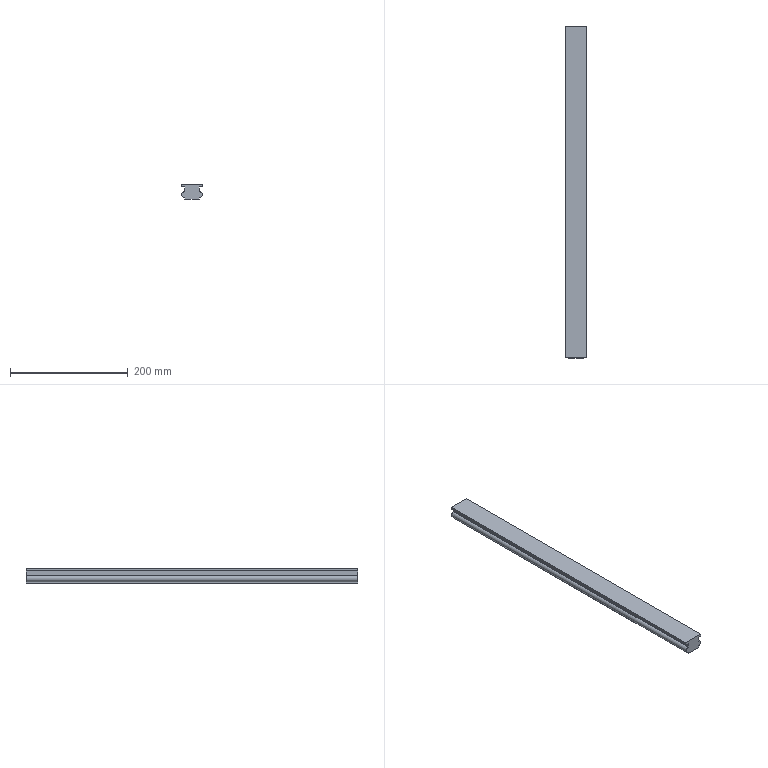Part | SolidWorks | features Extrusion 1 | 1 solid | 14 faces | box 36 x 563 x 25 mm | volume 420865 mm3 | plane 12 | cylinder 2 | commonest cylinder face diameters 10 x2
STEP:
#1=CARTESIAN_POINT('',(12.5,0.,5.));
#2=VERTEX_POINT('',#1);
#3=CARTESIAN_POINT('',(12.5,0.,-5.));
#4=VERTEX_POINT('',#3);
#5=CARTESIAN_POINT('',(12.5,0.,0.));
#6=DIRECTION('',(0.,1.,0.));
#7=DIRECTION('',(0.,0.,1.));
#8=AXIS2_PLACEMENT_3D('',#5,#6,#7);
#9=CIRCLE('',#8,5.);
#10=EDGE_CURVE('',#2,#4,#9,.T.);
#11=ORIENTED_EDGE('',*,*,#10,.T.);
#12=CARTESIAN_POINT('',(12.5,563.,-5.));
#13=VERTEX_POINT('',#12);
#14=CARTESIAN_POINT('',(12.5,563.,-5.));
#15=DIRECTION('',(0.,-1.,0.));
#16=VECTOR('',#15,1000.);
#17=LINE('',#14,#16);
#18=EDGE_CURVE('',#13,#4,#17,.T.);
#19=ORIENTED_EDGE('',*,*,#18,.F.);
#20=CARTESIAN_POINT('',(12.5,563.,5.));
#21=VERTEX_POINT('',#20);
#22=CARTESIAN_POINT('',(12.5,563.,0.));
#23=DIRECTION('',(0.,1.,0.));
#24=DIRECTION('',(0.,0.,1.));
#25=AXIS2_PLACEMENT_3D('',#22,#23,#24);
#26=CIRCLE('',#25,5.);
#27=EDGE_CURVE('',#21,#13,#26,.T.);
#28=ORIENTED_EDGE('',*,*,#27,.F.);
#29=CARTESIAN_POINT('',(12.5,563.,5.));
#30=DIRECTION('',(0.,-1.,0.));
#31=VECTOR('',#30,1000.);
#32=LINE('',#29,#31);
#33=EDGE_CURVE('',#21,#2,#32,.T.);
#34=ORIENTED_EDGE('',*,*,#33,.T.);
#35=EDGE_LOOP('',(#11,#19,#28,#34));
#36=FACE_OUTER_BOUND('',#35,.T.);
#37=CARTESIAN_POINT('',(12.5,563.,0.));
#38=DIRECTION('',(0.,-1.,0.));
#39=DIRECTION('',(0.,0.,-1.));
#40=AXIS2_PLACEMENT_3D('',#37,#38,#39);
#41=CYLINDRICAL_SURFACE('',#40,5.);
#42=ADVANCED_FACE('',(#36),#41,.T.);
#43=CARTESIAN_POINT('',(12.5,0.,-8.));
#44=VERTEX_POINT('',#43);
#45=CARTESIAN_POINT('',(12.5,0.,-8.));
#46=DIRECTION('',(0.,0.,-1.));
#47=VECTOR('',#46,1000.);
#48=LINE('',#45,#47);
#49=EDGE_CURVE('',#4,#44,#48,.T.);
#50=ORIENTED_EDGE('',*,*,#49,.T.);
#51=CARTESIAN_POINT('',(12.5,563.,-8.));
#52=VERTEX_POINT('',#51);
#53=CARTESIAN_POINT('',(12.5,563.,-8.));
#54=DIRECTION('',(0.,-1.,0.));
#55=VECTOR('',#54,1000.);
#56=LINE('',#53,#55);
#57=EDGE_CURVE('',#52,#44,#56,.T.);
#58=ORIENTED_EDGE('',*,*,#57,.F.);
#59=CARTESIAN_POINT('',(12.5,563.,-8.));
#60=DIRECTION('',(0.,0.,-1.));
#61=VECTOR('',#60,1000.);
#62=LINE('',#59,#61);
#63=EDGE_CURVE('',#13,#52,#62,.T.);
#64=ORIENTED_EDGE('',*,*,#63,.F.);
#65=ORIENTED_EDGE('',*,*,#18,.T.);
#66=EDGE_LOOP('',(#50,#58,#64,#65));
#67=FACE_OUTER_BOUND('',#66,.T.);
#68=CARTESIAN_POINT('',(12.5,563.,-8.));
#69=DIRECTION('',(-1.,0.,0.));
#70=DIRECTION('',(0.,0.,1.));
#71=AXIS2_PLACEMENT_3D('',#68,#69,#70);
#72=PLANE('',#71);
#73=ADVANCED_FACE('',(#67),#72,.F.);
#74=CARTESIAN_POINT('',(-12.5,0.,-8.));
#75=VERTEX_POINT('',#74);
#76=CARTESIAN_POINT('',(-12.5,0.,-8.));
#77=DIRECTION('',(-1.,0.,0.));
#78=VECTOR('',#77,1000.);
#79=LINE('',#76,#78);
#80=EDGE_CURVE('',#44,#75,#79,.T.);
#81=ORIENTED_EDGE('',*,*,#80,.T.);
#82=CARTESIAN_POINT('',(-12.5,563.,-8.));
#83=VERTEX_POINT('',#82);
#84=CARTESIAN_POINT('',(-12.5,563.,-8.));
#85=DIRECTION('',(0.,-1.,0.));
#86=VECTOR('',#85,1000.);
#87=LINE('',#84,#86);
#88=EDGE_CURVE('',#83,#75,#87,.T.);
#89=ORIENTED_EDGE('',*,*,#88,.F.);
#90=CARTESIAN_POINT('',(-12.5,563.,-8.));
#91=DIRECTION('',(-1.,0.,0.));
#92=VECTOR('',#91,1000.);
#93=LINE('',#90,#92);
#94=EDGE_CURVE('',#52,#83,#93,.T.);
#95=ORIENTED_EDGE('',*,*,#94,.F.);
#96=ORIENTED_EDGE('',*,*,#57,.T.);
#97=EDGE_LOOP('',(#81,#89,#95,#96));
#98=FACE_OUTER_BOUND('',#97,.T.);
#99=CARTESIAN_POINT('',(-12.5,563.,-8.));
#100=DIRECTION('',(0.,0.,1.));
#101=DIRECTION('',(1.,0.,0.));
#102=AXIS2_PLACEMENT_3D('',#99,#100,#101);
#103=PLANE('',#102);
#104=ADVANCED_FACE('',(#98),#103,.F.);
#105=CARTESIAN_POINT('',(-12.5,0.,-5.));
#106=VERTEX_POINT('',#105);
#107=CARTESIAN_POINT('',(-12.5,0.,-5.));
#108=DIRECTION('',(0.,0.,1.));
#109=VECTOR('',#108,1000.);
#110=LINE('',#107,#109);
#111=EDGE_CURVE('',#75,#106,#110,.T.);
#112=ORIENTED_EDGE('',*,*,#111,.T.);
#113=CARTESIAN_POINT('',(-12.5,563.,-5.));
#114=VERTEX_POINT('',#113);
#115=CARTESIAN_POINT('',(-12.5,563.,-5.));
#116=DIRECTION('',(0.,-1.,0.));
#117=VECTOR('',#116,1000.);
#118=LINE('',#115,#117);
#119=EDGE_CURVE('',#114,#106,#118,.T.);
#120=ORIENTED_EDGE('',*,*,#119,.F.);
#121=CARTESIAN_POINT('',(-12.5,563.,-5.));
#122=DIRECTION('',(0.,0.,1.));
#123=VECTOR('',#122,1000.);
#124=LINE('',#121,#123);
#125=EDGE_CURVE('',#83,#114,#124,.T.);
#126=ORIENTED_EDGE('',*,*,#125,.F.);
#127=ORIENTED_EDGE('',*,*,#88,.T.);
#128=EDGE_LOOP('',(#112,#120,#126,#127));
#129=FACE_OUTER_BOUND('',#128,.T.);
#130=CARTESIAN_POINT('',(-12.5,563.,-5.));
#131=DIRECTION('',(1.,0.,0.));
#132=DIRECTION('',(0.,0.,-1.));
#133=AXIS2_PLACEMENT_3D('',#130,#131,#132);
#134=PLANE('',#133);
#135=ADVANCED_FACE('',(#129),#134,.F.);
#136=CARTESIAN_POINT('',(-12.5,0.,5.));
#137=VERTEX_POINT('',#136);
#138=CARTESIAN_POINT('',(-12.5,0.,0.));
#139=DIRECTION('',(0.,1.,0.));
#140=DIRECTION('',(0.,0.,1.));
#141=AXIS2_PLACEMENT_3D('',#138,#139,#140);
#142=CIRCLE('',#141,5.);
#143=EDGE_CURVE('',#106,#137,#142,.T.);
#144=ORIENTED_EDGE('',*,*,#143,.T.);
#145=CARTESIAN_POINT('',(-12.5,563.,5.));
#146=VERTEX_POINT('',#145);
#147=CARTESIAN_POINT('',(-12.5,563.,5.));
#148=DIRECTION('',(0.,-1.,0.));
#149=VECTOR('',#148,1000.);
#150=LINE('',#147,#149);
#151=EDGE_CURVE('',#146,#137,#150,.T.);
#152=ORIENTED_EDGE('',*,*,#151,.F.);
#153=CARTESIAN_POINT('',(-12.5,563.,0.));
#154=DIRECTION('',(0.,1.,0.));
#155=DIRECTION('',(0.,0.,1.));
#156=AXIS2_PLACEMENT_3D('',#153,#154,#155);
#157=CIRCLE('',#156,5.);
#158=EDGE_CURVE('',#114,#146,#157,.T.);
#159=ORIENTED_EDGE('',*,*,#158,.F.);
#160=ORIENTED_EDGE('',*,*,#119,.T.);
#161=EDGE_LOOP('',(#144,#152,#159,#160));
#162=FACE_OUTER_BOUND('',#161,.T.);
#163=CARTESIAN_POINT('',(-12.5,563.,0.));
#164=DIRECTION('',(0.,-1.,0.));
#165=DIRECTION('',(0.,0.,-1.));
#166=AXIS2_PLACEMENT_3D('',#163,#164,#165);
#167=CYLINDRICAL_SURFACE('',#166,5.);
#168=ADVANCED_FACE('',(#162),#167,.T.);
#169=CARTESIAN_POINT('',(-12.5,0.,13.));
#170=VERTEX_POINT('',#169);
#171=CARTESIAN_POINT('',(-12.5,0.,5.));
#172=DIRECTION('',(0.,0.,1.));
#173=VECTOR('',#172,1000.);
#174=LINE('',#171,#173);
#175=EDGE_CURVE('',#137,#170,#174,.T.);
#176=ORIENTED_EDGE('',*,*,#175,.T.);
#177=CARTESIAN_POINT('',(-12.5,563.,13.));
#178=VERTEX_POINT('',#177);
#179=CARTESIAN_POINT('',(-12.5,563.,13.));
#180=DIRECTION('',(0.,-1.,0.));
#181=VECTOR('',#180,1000.);
#182=LINE('',#179,#181);
#183=EDGE_CURVE('',#178,#170,#182,.T.);
#184=ORIENTED_EDGE('',*,*,#183,.F.);
#185=CARTESIAN_POINT('',(-12.5,563.,5.));
#186=DIRECTION('',(0.,0.,1.));
#187=VECTOR('',#186,1000.);
#188=LINE('',#185,#187);
#189=EDGE_CURVE('',#146,#178,#188,.T.);
#190=ORIENTED_EDGE('',*,*,#189,.F.);
#191=ORIENTED_EDGE('',*,*,#151,.T.);
#192=EDGE_LOOP('',(#176,#184,#190,#191));
#193=FACE_OUTER_BOUND('',#192,.T.);
#194=CARTESIAN_POINT('',(-12.5,563.,5.));
#195=DIRECTION('',(1.,0.,0.));
#196=DIRECTION('',(0.,0.,-1.));
#197=AXIS2_PLACEMENT_3D('',#194,#195,#196);
#198=PLANE('',#197);
#199=ADVANCED_FACE('',(#193),#198,.F.);
#200=CARTESIAN_POINT('',(-18.,0.,13.));
#201=VERTEX_POINT('',#200);
#202=CARTESIAN_POINT('',(-12.5,0.,13.));
#203=DIRECTION('',(-1.,0.,0.));
#204=VECTOR('',#203,1000.);
#205=LINE('',#202,#204);
#206=EDGE_CURVE('',#170,#201,#205,.T.);
#207=ORIENTED_EDGE('',*,*,#206,.T.);
#208=CARTESIAN_POINT('',(-18.,563.,13.));
#209=VERTEX_POINT('',#208);
#210=CARTESIAN_POINT('',(-18.,563.,13.));
#211=DIRECTION('',(0.,-1.,0.));
#212=VECTOR('',#211,1000.);
#213=LINE('',#210,#212);
#214=EDGE_CURVE('',#209,#201,#213,.T.);
#215=ORIENTED_EDGE('',*,*,#214,.F.);
#216=CARTESIAN_POINT('',(-12.5,563.,13.));
#217=DIRECTION('',(-1.,0.,0.));
#218=VECTOR('',#217,1000.);
#219=LINE('',#216,#218);
#220=EDGE_CURVE('',#178,#209,#219,.T.);
#221=ORIENTED_EDGE('',*,*,#220,.F.);
#222=ORIENTED_EDGE('',*,*,#183,.T.);
#223=EDGE_LOOP('',(#207,#215,#221,#222));
#224=FACE_OUTER_BOUND('',#223,.T.);
#225=CARTESIAN_POINT('',(-12.5,563.,13.));
#226=DIRECTION('',(0.,0.,1.));
#227=DIRECTION('',(1.,0.,0.));
#228=AXIS2_PLACEMENT_3D('',#225,#226,#227);
#229=PLANE('',#228);
#230=ADVANCED_FACE('',(#224),#229,.F.);
#231=CARTESIAN_POINT('',(-18.,0.,17.));
#232=VERTEX_POINT('',#231);
#233=CARTESIAN_POINT('',(-18.,0.,13.));
#234=DIRECTION('',(0.,0.,1.));
#235=VECTOR('',#234,1000.);
#236=LINE('',#233,#235);
#237=EDGE_CURVE('',#201,#232,#236,.T.);
#238=ORIENTED_EDGE('',*,*,#237,.T.);
#239=CARTESIAN_POINT('',(-18.,563.,17.));
#240=VERTEX_POINT('',#239);
#241=CARTESIAN_POINT('',(-18.,563.,17.));
#242=DIRECTION('',(0.,-1.,0.));
#243=VECTOR('',#242,1000.);
#244=LINE('',#241,#243);
#245=EDGE_CURVE('',#240,#232,#244,.T.);
#246=ORIENTED_EDGE('',*,*,#245,.F.);
#247=CARTESIAN_POINT('',(-18.,563.,13.));
#248=DIRECTION('',(0.,0.,1.));
#249=VECTOR('',#248,1000.);
#250=LINE('',#247,#249);
#251=EDGE_CURVE('',#209,#240,#250,.T.);
#252=ORIENTED_EDGE('',*,*,#251,.F.);
#253=ORIENTED_EDGE('',*,*,#214,.T.);
#254=EDGE_LOOP('',(#238,#246,#252,#253));
#255=FACE_OUTER_BOUND('',#254,.T.);
#256=CARTESIAN_POINT('',(-18.,563.,13.));
#257=DIRECTION('',(1.,0.,0.));
#258=DIRECTION('',(0.,0.,-1.));
#259=AXIS2_PLACEMENT_3D('',#256,#257,#258);
#260=PLANE('',#259);
#261=ADVANCED_FACE('',(#255),#260,.F.);
#262=CARTESIAN_POINT('',(18.,0.,17.));
#263=VERTEX_POINT('',#262);
#264=CARTESIAN_POINT('',(-18.,0.,17.));
#265=DIRECTION('',(1.,0.,0.));
#266=VECTOR('',#265,1000.);
#267=LINE('',#264,#266);
#268=EDGE_CURVE('',#232,#263,#267,.T.);
#269=ORIENTED_EDGE('',*,*,#268,.T.);
#270=CARTESIAN_POINT('',(18.,563.,17.));
#271=VERTEX_POINT('',#270);
#272=CARTESIAN_POINT('',(18.,563.,17.));
#273=DIRECTION('',(0.,-1.,0.));
#274=VECTOR('',#273,1000.);
#275=LINE('',#272,#274);
#276=EDGE_CURVE('',#271,#263,#275,.T.);
#277=ORIENTED_EDGE('',*,*,#276,.F.);
#278=CARTESIAN_POINT('',(-18.,563.,17.));
#279=DIRECTION('',(1.,0.,0.));
#280=VECTOR('',#279,1000.);
#281=LINE('',#278,#280);
#282=EDGE_CURVE('',#240,#271,#281,.T.);
#283=ORIENTED_EDGE('',*,*,#282,.F.);
#284=ORIENTED_EDGE('',*,*,#245,.T.);
#285=EDGE_LOOP('',(#269,#277,#283,#284));
#286=FACE_OUTER_BOUND('',#285,.T.);
#287=CARTESIAN_POINT('',(-18.,563.,17.));
#288=DIRECTION('',(0.,0.,-1.));
#289=DIRECTION('',(-1.,0.,0.));
#290=AXIS2_PLACEMENT_3D('',#287,#288,#289);
#291=PLANE('',#290);
#292=ADVANCED_FACE('',(#286),#291,.F.);
#293=CARTESIAN_POINT('',(18.,0.,13.));
#294=VERTEX_POINT('',#293);
#295=CARTESIAN_POINT('',(18.,0.,17.));
#296=DIRECTION('',(0.,0.,-1.));
#297=VECTOR('',#296,1000.);
#298=LINE('',#295,#297);
#299=EDGE_CURVE('',#263,#294,#298,.T.);
#300=ORIENTED_EDGE('',*,*,#299,.T.);
#301=CARTESIAN_POINT('',(18.,563.,13.));
#302=VERTEX_POINT('',#301);
#303=CARTESIAN_POINT('',(18.,563.,13.));
#304=DIRECTION('',(0.,-1.,0.));
#305=VECTOR('',#304,1000.);
#306=LINE('',#303,#305);
#307=EDGE_CURVE('',#302,#294,#306,.T.);
#308=ORIENTED_EDGE('',*,*,#307,.F.);
#309=CARTESIAN_POINT('',(18.,563.,17.));
#310=DIRECTION('',(0.,0.,-1.));
#311=VECTOR('',#310,1000.);
#312=LINE('',#309,#311);
#313=EDGE_CURVE('',#271,#302,#312,.T.);
#314=ORIENTED_EDGE('',*,*,#313,.F.);
#315=ORIENTED_EDGE('',*,*,#276,.T.);
#316=EDGE_LOOP('',(#300,#308,#314,#315));
#317=FACE_OUTER_BOUND('',#316,.T.);
#318=CARTESIAN_POINT('',(18.,563.,17.));
#319=DIRECTION('',(-1.,0.,0.));
#320=DIRECTION('',(0.,0.,1.));
#321=AXIS2_PLACEMENT_3D('',#318,#319,#320);
#322=PLANE('',#321);
#323=ADVANCED_FACE('',(#317),#322,.F.);
#324=CARTESIAN_POINT('',(12.5,0.,13.));
#325=VERTEX_POINT('',#324);
#326=CARTESIAN_POINT('',(18.,0.,13.));
#327=DIRECTION('',(-1.,0.,0.));
#328=VECTOR('',#327,1000.);
#329=LINE('',#326,#328);
#330=EDGE_CURVE('',#294,#325,#329,.T.);
#331=ORIENTED_EDGE('',*,*,#330,.T.);
#332=CARTESIAN_POINT('',(12.5,563.,13.));
#333=VERTEX_POINT('',#332);
#334=CARTESIAN_POINT('',(12.5,563.,13.));
#335=DIRECTION('',(0.,-1.,0.));
#336=VECTOR('',#335,1000.);
#337=LINE('',#334,#336);
#338=EDGE_CURVE('',#333,#325,#337,.T.);
#339=ORIENTED_EDGE('',*,*,#338,.F.);
#340=CARTESIAN_POINT('',(18.,563.,13.));
#341=DIRECTION('',(-1.,0.,0.));
#342=VECTOR('',#341,1000.);
#343=LINE('',#340,#342);
#344=EDGE_CURVE('',#302,#333,#343,.T.);
#345=ORIENTED_EDGE('',*,*,#344,.F.);
#346=ORIENTED_EDGE('',*,*,#307,.T.);
#347=EDGE_LOOP('',(#331,#339,#345,#346));
#348=FACE_OUTER_BOUND('',#347,.T.);
#349=CARTESIAN_POINT('',(18.,563.,13.));
#350=DIRECTION('',(0.,0.,1.));
#351=DIRECTION('',(1.,0.,0.));
#352=AXIS2_PLACEMENT_3D('',#349,#350,#351);
#353=PLANE('',#352);
#354=ADVANCED_FACE('',(#348),#353,.F.);
#355=CARTESIAN_POINT('',(12.5,0.,13.));
#356=DIRECTION('',(0.,0.,-1.));
#357=VECTOR('',#356,1000.);
#358=LINE('',#355,#357);
#359=EDGE_CURVE('',#325,#2,#358,.T.);
#360=ORIENTED_EDGE('',*,*,#359,.T.);
#361=ORIENTED_EDGE('',*,*,#33,.F.);
#362=CARTESIAN_POINT('',(12.5,563.,13.));
#363=DIRECTION('',(0.,0.,-1.));
#364=VECTOR('',#363,1000.);
#365=LINE('',#362,#364);
#366=EDGE_CURVE('',#333,#21,#365,.T.);
#367=ORIENTED_EDGE('',*,*,#366,.F.);
#368=ORIENTED_EDGE('',*,*,#338,.T.);
#369=EDGE_LOOP('',(#360,#361,#367,#368));
#370=FACE_OUTER_BOUND('',#369,.T.);
#371=CARTESIAN_POINT('',(12.5,563.,13.));
#372=DIRECTION('',(-1.,0.,0.));
#373=DIRECTION('',(0.,0.,1.));
#374=AXIS2_PLACEMENT_3D('',#371,#372,#373);
#375=PLANE('',#374);
#376=ADVANCED_FACE('',(#370),#375,.F.);
#377=ORIENTED_EDGE('',*,*,#27,.T.);
#378=ORIENTED_EDGE('',*,*,#63,.T.);
#379=ORIENTED_EDGE('',*,*,#94,.T.);
#380=ORIENTED_EDGE('',*,*,#125,.T.);
#381=ORIENTED_EDGE('',*,*,#158,.T.);
#382=ORIENTED_EDGE('',*,*,#189,.T.);
#383=ORIENTED_EDGE('',*,*,#220,.T.);
#384=ORIENTED_EDGE('',*,*,#251,.T.);
#385=ORIENTED_EDGE('',*,*,#282,.T.);
#386=ORIENTED_EDGE('',*,*,#313,.T.);
#387=ORIENTED_EDGE('',*,*,#344,.T.);
#388=ORIENTED_EDGE('',*,*,#366,.T.);
#389=EDGE_LOOP('',(#377,#378,#379,#380,#381,#382,#383,#384,#385,#386,#387,#388));
#390=FACE_OUTER_BOUND('',#389,.T.);
#391=CARTESIAN_POINT('',(12.5,563.,0.));
#392=DIRECTION('',(0.,1.,0.));
#393=DIRECTION('',(0.,0.,1.));
#394=AXIS2_PLACEMENT_3D('',#391,#392,#393);
#395=PLANE('',#394);
#396=ADVANCED_FACE('',(#390),#395,.T.);
#397=ORIENTED_EDGE('',*,*,#10,.F.);
#398=ORIENTED_EDGE('',*,*,#359,.F.);
#399=ORIENTED_EDGE('',*,*,#330,.F.);
#400=ORIENTED_EDGE('',*,*,#299,.F.);
#401=ORIENTED_EDGE('',*,*,#268,.F.);
#402=ORIENTED_EDGE('',*,*,#237,.F.);
#403=ORIENTED_EDGE('',*,*,#206,.F.);
#404=ORIENTED_EDGE('',*,*,#175,.F.);
#405=ORIENTED_EDGE('',*,*,#143,.F.);
#406=ORIENTED_EDGE('',*,*,#111,.F.);
#407=ORIENTED_EDGE('',*,*,#80,.F.);
#408=ORIENTED_EDGE('',*,*,#49,.F.);
#409=EDGE_LOOP('',(#397,#398,#399,#400,#401,#402,#403,#404,#405,#406,#407,#408));
#410=FACE_OUTER_BOUND('',#409,.T.);
#411=CARTESIAN_POINT('',(12.5,0.,0.));
#412=DIRECTION('',(0.,1.,0.));
#413=DIRECTION('',(0.,0.,1.));
#414=AXIS2_PLACEMENT_3D('',#411,#412,#413);
#415=PLANE('',#414);
#416=ADVANCED_FACE('',(#410),#415,.F.);
#417=CLOSED_SHELL('',(#42,#73,#104,#135,#168,#199,#230,#261,#292,#323,#354,#376,#396,#416));
#418=MANIFOLD_SOLID_BREP('',#417);
#419=CARTESIAN_POINT('',(0.,0.,0.));
#420=DIRECTION('',(0.,0.,1.));
#421=DIRECTION('',(1.,0.,0.));
#422=AXIS2_PLACEMENT_3D('',#419,#420,#421);
#423=(LENGTH_UNIT()NAMED_UNIT(*)SI_UNIT(.MILLI.,.METRE.));
#424=UNCERTAINTY_MEASURE_WITH_UNIT(LENGTH_MEASURE(0.00001),#423,'','');
#425=(NAMED_UNIT(*)PLANE_ANGLE_UNIT()SI_UNIT($,.RADIAN.));
#426=(NAMED_UNIT(*)SI_UNIT($,.STERADIAN.)SOLID_ANGLE_UNIT());
#427=(GEOMETRIC_REPRESENTATION_CONTEXT(3)GLOBAL_UNCERTAINTY_ASSIGNED_CONTEXT((#424))GLOBAL_UNIT_ASSIGNED_CONTEXT((#423,#425,#426))REPRESENTATION_CONTEXT('',''));
#428=ADVANCED_BREP_SHAPE_REPRESENTATION('',(#418,#422),#427);